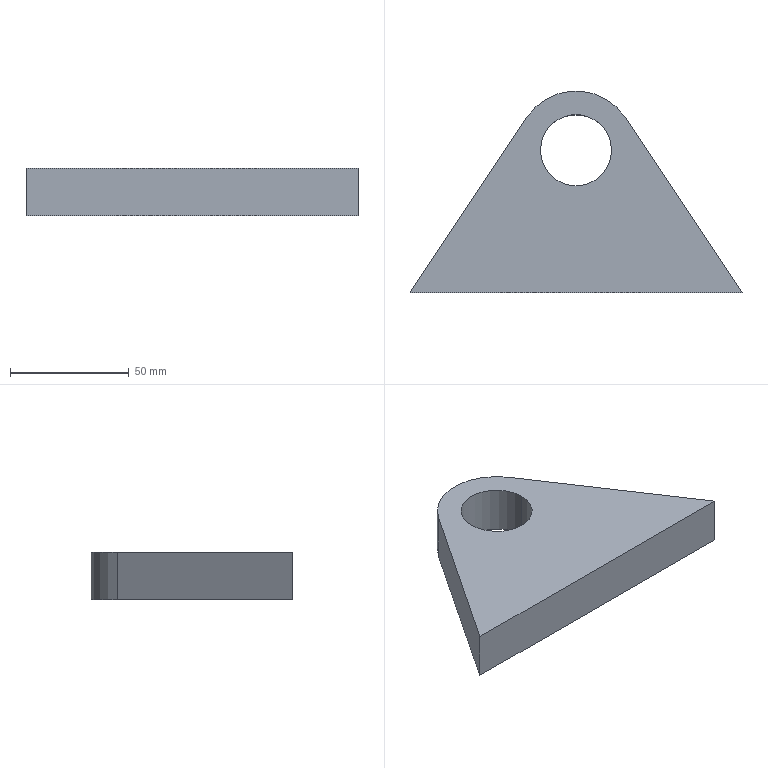Part | SolidWorks | features BaseBody 1 | 1 solid | 8 faces | box 140 x 85 x 20 mm | volume 126524 mm3 | plane 5 | cylinder 3 | commonest cylinder face diameters 30 x2 50 x1
STEP:
#1=CARTESIAN_POINT('',(2539.523,1394.061,20.));
#2=VERTEX_POINT('',#1);
#3=CARTESIAN_POINT('',(2569.523,1394.061,20.));
#4=VERTEX_POINT('',#3);
#5=CARTESIAN_POINT('',(2554.523,1394.061,20.));
#6=DIRECTION('',(0.,0.,1.));
#7=DIRECTION('',(1.,0.,0.));
#8=AXIS2_PLACEMENT_3D('',#5,#6,#7);
#9=CIRCLE('',#8,15.);
#10=EDGE_CURVE('',#2,#4,#9,.T.);
#11=ORIENTED_EDGE('',*,*,#10,.T.);
#12=CARTESIAN_POINT('',(2569.523,1394.061,0.));
#13=VERTEX_POINT('',#12);
#14=CARTESIAN_POINT('',(2569.523,1394.061,20.));
#15=DIRECTION('',(0.,0.,-1.));
#16=VECTOR('',#15,1000.);
#17=LINE('',#14,#16);
#18=EDGE_CURVE('',#4,#13,#17,.T.);
#19=ORIENTED_EDGE('',*,*,#18,.T.);
#20=CARTESIAN_POINT('',(2539.523,1394.061,0.));
#21=VERTEX_POINT('',#20);
#22=CARTESIAN_POINT('',(2554.523,1394.061,0.));
#23=DIRECTION('',(0.,0.,1.));
#24=DIRECTION('',(1.,0.,0.));
#25=AXIS2_PLACEMENT_3D('',#22,#23,#24);
#26=CIRCLE('',#25,15.);
#27=EDGE_CURVE('',#21,#13,#26,.T.);
#28=ORIENTED_EDGE('',*,*,#27,.F.);
#29=CARTESIAN_POINT('',(2539.523,1394.061,20.));
#30=DIRECTION('',(0.,0.,-1.));
#31=VECTOR('',#30,1000.);
#32=LINE('',#29,#31);
#33=EDGE_CURVE('',#2,#21,#32,.T.);
#34=ORIENTED_EDGE('',*,*,#33,.F.);
#35=EDGE_LOOP('',(#11,#19,#28,#34));
#36=FACE_OUTER_BOUND('',#35,.T.);
#37=CARTESIAN_POINT('',(2554.523,1394.061,20.));
#38=DIRECTION('',(0.,0.,-1.));
#39=DIRECTION('',(-1.,0.,0.));
#40=AXIS2_PLACEMENT_3D('',#37,#38,#39);
#41=CYLINDRICAL_SURFACE('',#40,15.);
#42=ADVANCED_FACE('',(#36),#41,.F.);
#43=CARTESIAN_POINT('',(2575.33,1407.919,20.));
#44=VERTEX_POINT('',#43);
#45=CARTESIAN_POINT('',(2533.715,1407.919,20.));
#46=VERTEX_POINT('',#45);
#47=CARTESIAN_POINT('',(2554.523,1394.061,20.));
#48=DIRECTION('',(0.,0.,1.));
#49=DIRECTION('',(1.,0.,0.));
#50=AXIS2_PLACEMENT_3D('',#47,#48,#49);
#51=CIRCLE('',#50,25.);
#52=EDGE_CURVE('',#44,#46,#51,.T.);
#53=ORIENTED_EDGE('',*,*,#52,.T.);
#54=CARTESIAN_POINT('',(2484.523,1334.061,20.));
#55=VERTEX_POINT('',#54);
#56=CARTESIAN_POINT('',(2533.715,1407.919,20.));
#57=DIRECTION('',(-0.5543,-0.8323,0.));
#58=VECTOR('',#57,1000.);
#59=LINE('',#56,#58);
#60=EDGE_CURVE('',#46,#55,#59,.T.);
#61=ORIENTED_EDGE('',*,*,#60,.T.);
#62=CARTESIAN_POINT('',(2624.523,1334.061,20.));
#63=VERTEX_POINT('',#62);
#64=CARTESIAN_POINT('',(2484.523,1334.061,20.));
#65=DIRECTION('',(1.,0.,0.));
#66=VECTOR('',#65,1000.);
#67=LINE('',#64,#66);
#68=EDGE_CURVE('',#55,#63,#67,.T.);
#69=ORIENTED_EDGE('',*,*,#68,.T.);
#70=CARTESIAN_POINT('',(2575.33,1407.919,20.));
#71=DIRECTION('',(-0.5543,0.8323,0.));
#72=VECTOR('',#71,1000.);
#73=LINE('',#70,#72);
#74=EDGE_CURVE('',#63,#44,#73,.T.);
#75=ORIENTED_EDGE('',*,*,#74,.T.);
#76=EDGE_LOOP('',(#53,#61,#69,#75));
#77=FACE_OUTER_BOUND('',#76,.T.);
#78=ORIENTED_EDGE('',*,*,#10,.F.);
#79=CARTESIAN_POINT('',(2554.523,1394.061,20.));
#80=DIRECTION('',(0.,0.,1.));
#81=DIRECTION('',(1.,0.,0.));
#82=AXIS2_PLACEMENT_3D('',#79,#80,#81);
#83=CIRCLE('',#82,15.);
#84=EDGE_CURVE('',#4,#2,#83,.T.);
#85=ORIENTED_EDGE('',*,*,#84,.F.);
#86=EDGE_LOOP('',(#78,#85));
#87=FACE_BOUND('',#86,.T.);
#88=CARTESIAN_POINT('',(2554.523,1394.061,20.));
#89=DIRECTION('',(0.,0.,1.));
#90=DIRECTION('',(1.,0.,0.));
#91=AXIS2_PLACEMENT_3D('',#88,#89,#90);
#92=PLANE('',#91);
#93=ADVANCED_FACE('',(#77,#87),#92,.T.);
#94=CARTESIAN_POINT('',(2575.33,1407.919,0.));
#95=VERTEX_POINT('',#94);
#96=CARTESIAN_POINT('',(2533.715,1407.919,0.));
#97=VERTEX_POINT('',#96);
#98=CARTESIAN_POINT('',(2554.523,1394.061,0.));
#99=DIRECTION('',(0.,0.,1.));
#100=DIRECTION('',(1.,0.,0.));
#101=AXIS2_PLACEMENT_3D('',#98,#99,#100);
#102=CIRCLE('',#101,25.);
#103=EDGE_CURVE('',#95,#97,#102,.T.);
#104=ORIENTED_EDGE('',*,*,#103,.F.);
#105=CARTESIAN_POINT('',(2624.523,1334.061,0.));
#106=VERTEX_POINT('',#105);
#107=CARTESIAN_POINT('',(2575.33,1407.919,0.));
#108=DIRECTION('',(-0.5543,0.8323,0.));
#109=VECTOR('',#108,1000.);
#110=LINE('',#107,#109);
#111=EDGE_CURVE('',#106,#95,#110,.T.);
#112=ORIENTED_EDGE('',*,*,#111,.F.);
#113=CARTESIAN_POINT('',(2484.523,1334.061,0.));
#114=VERTEX_POINT('',#113);
#115=CARTESIAN_POINT('',(2484.523,1334.061,0.));
#116=DIRECTION('',(1.,0.,0.));
#117=VECTOR('',#116,1000.);
#118=LINE('',#115,#117);
#119=EDGE_CURVE('',#114,#106,#118,.T.);
#120=ORIENTED_EDGE('',*,*,#119,.F.);
#121=CARTESIAN_POINT('',(2533.715,1407.919,0.));
#122=DIRECTION('',(-0.5543,-0.8323,0.));
#123=VECTOR('',#122,1000.);
#124=LINE('',#121,#123);
#125=EDGE_CURVE('',#97,#114,#124,.T.);
#126=ORIENTED_EDGE('',*,*,#125,.F.);
#127=EDGE_LOOP('',(#104,#112,#120,#126));
#128=FACE_OUTER_BOUND('',#127,.T.);
#129=ORIENTED_EDGE('',*,*,#27,.T.);
#130=CARTESIAN_POINT('',(2554.523,1394.061,0.));
#131=DIRECTION('',(0.,0.,1.));
#132=DIRECTION('',(1.,0.,0.));
#133=AXIS2_PLACEMENT_3D('',#130,#131,#132);
#134=CIRCLE('',#133,15.);
#135=EDGE_CURVE('',#13,#21,#134,.T.);
#136=ORIENTED_EDGE('',*,*,#135,.T.);
#137=EDGE_LOOP('',(#129,#136));
#138=FACE_BOUND('',#137,.T.);
#139=CARTESIAN_POINT('',(2554.523,1394.061,0.));
#140=DIRECTION('',(0.,0.,1.));
#141=DIRECTION('',(1.,0.,0.));
#142=AXIS2_PLACEMENT_3D('',#139,#140,#141);
#143=PLANE('',#142);
#144=ADVANCED_FACE('',(#128,#138),#143,.F.);
#145=ORIENTED_EDGE('',*,*,#103,.T.);
#146=CARTESIAN_POINT('',(2533.715,1407.919,20.));
#147=DIRECTION('',(0.,0.,-1.));
#148=VECTOR('',#147,1000.);
#149=LINE('',#146,#148);
#150=EDGE_CURVE('',#46,#97,#149,.T.);
#151=ORIENTED_EDGE('',*,*,#150,.F.);
#152=ORIENTED_EDGE('',*,*,#52,.F.);
#153=CARTESIAN_POINT('',(2575.33,1407.919,20.));
#154=DIRECTION('',(0.,0.,-1.));
#155=VECTOR('',#154,1000.);
#156=LINE('',#153,#155);
#157=EDGE_CURVE('',#44,#95,#156,.T.);
#158=ORIENTED_EDGE('',*,*,#157,.T.);
#159=EDGE_LOOP('',(#145,#151,#152,#158));
#160=FACE_OUTER_BOUND('',#159,.T.);
#161=CARTESIAN_POINT('',(2554.523,1394.061,20.));
#162=DIRECTION('',(0.,0.,-1.));
#163=DIRECTION('',(-1.,0.,0.));
#164=AXIS2_PLACEMENT_3D('',#161,#162,#163);
#165=CYLINDRICAL_SURFACE('',#164,25.);
#166=ADVANCED_FACE('',(#160),#165,.T.);
#167=ORIENTED_EDGE('',*,*,#125,.T.);
#168=CARTESIAN_POINT('',(2484.523,1334.061,20.));
#169=DIRECTION('',(0.,0.,-1.));
#170=VECTOR('',#169,1000.);
#171=LINE('',#168,#170);
#172=EDGE_CURVE('',#55,#114,#171,.T.);
#173=ORIENTED_EDGE('',*,*,#172,.F.);
#174=ORIENTED_EDGE('',*,*,#60,.F.);
#175=ORIENTED_EDGE('',*,*,#150,.T.);
#176=EDGE_LOOP('',(#167,#173,#174,#175));
#177=FACE_OUTER_BOUND('',#176,.T.);
#178=CARTESIAN_POINT('',(2533.715,1407.919,20.));
#179=DIRECTION('',(0.8323,-0.5543,0.));
#180=DIRECTION('',(0.5543,0.8323,0.));
#181=AXIS2_PLACEMENT_3D('',#178,#179,#180);
#182=PLANE('',#181);
#183=ADVANCED_FACE('',(#177),#182,.F.);
#184=ORIENTED_EDGE('',*,*,#119,.T.);
#185=CARTESIAN_POINT('',(2624.523,1334.061,20.));
#186=DIRECTION('',(0.,0.,-1.));
#187=VECTOR('',#186,1000.);
#188=LINE('',#185,#187);
#189=EDGE_CURVE('',#63,#106,#188,.T.);
#190=ORIENTED_EDGE('',*,*,#189,.F.);
#191=ORIENTED_EDGE('',*,*,#68,.F.);
#192=ORIENTED_EDGE('',*,*,#172,.T.);
#193=EDGE_LOOP('',(#184,#190,#191,#192));
#194=FACE_OUTER_BOUND('',#193,.T.);
#195=CARTESIAN_POINT('',(2484.523,1334.061,20.));
#196=DIRECTION('',(0.,1.,0.));
#197=DIRECTION('',(0.,0.,1.));
#198=AXIS2_PLACEMENT_3D('',#195,#196,#197);
#199=PLANE('',#198);
#200=ADVANCED_FACE('',(#194),#199,.F.);
#201=ORIENTED_EDGE('',*,*,#111,.T.);
#202=ORIENTED_EDGE('',*,*,#157,.F.);
#203=ORIENTED_EDGE('',*,*,#74,.F.);
#204=ORIENTED_EDGE('',*,*,#189,.T.);
#205=EDGE_LOOP('',(#201,#202,#203,#204));
#206=FACE_OUTER_BOUND('',#205,.T.);
#207=CARTESIAN_POINT('',(2575.33,1407.919,20.));
#208=DIRECTION('',(-0.8323,-0.5543,0.));
#209=DIRECTION('',(0.5543,-0.8323,0.));
#210=AXIS2_PLACEMENT_3D('',#207,#208,#209);
#211=PLANE('',#210);
#212=ADVANCED_FACE('',(#206),#211,.F.);
#213=ORIENTED_EDGE('',*,*,#18,.F.);
#214=ORIENTED_EDGE('',*,*,#84,.T.);
#215=ORIENTED_EDGE('',*,*,#33,.T.);
#216=ORIENTED_EDGE('',*,*,#135,.F.);
#217=EDGE_LOOP('',(#213,#214,#215,#216));
#218=FACE_OUTER_BOUND('',#217,.T.);
#219=CARTESIAN_POINT('',(2554.523,1394.061,20.));
#220=DIRECTION('',(0.,0.,-1.));
#221=DIRECTION('',(-1.,0.,0.));
#222=AXIS2_PLACEMENT_3D('',#219,#220,#221);
#223=CYLINDRICAL_SURFACE('',#222,15.);
#224=ADVANCED_FACE('',(#218),#223,.F.);
#225=CLOSED_SHELL('',(#42,#93,#144,#166,#183,#200,#212,#224));
#226=MANIFOLD_SOLID_BREP('',#225);
#227=CARTESIAN_POINT('',(0.,0.,0.));
#228=DIRECTION('',(0.,0.,1.));
#229=DIRECTION('',(1.,0.,0.));
#230=AXIS2_PLACEMENT_3D('',#227,#228,#229);
#231=(LENGTH_UNIT()NAMED_UNIT(*)SI_UNIT(.MILLI.,.METRE.));
#232=UNCERTAINTY_MEASURE_WITH_UNIT(LENGTH_MEASURE(0.00001),#231,'','');
#233=(NAMED_UNIT(*)PLANE_ANGLE_UNIT()SI_UNIT($,.RADIAN.));
#234=(NAMED_UNIT(*)SI_UNIT($,.STERADIAN.)SOLID_ANGLE_UNIT());
#235=(GEOMETRIC_REPRESENTATION_CONTEXT(3)GLOBAL_UNCERTAINTY_ASSIGNED_CONTEXT((#232))GLOBAL_UNIT_ASSIGNED_CONTEXT((#231,#233,#234))REPRESENTATION_CONTEXT('',''));
#236=ADVANCED_BREP_SHAPE_REPRESENTATION('',(#226,#230),#235);